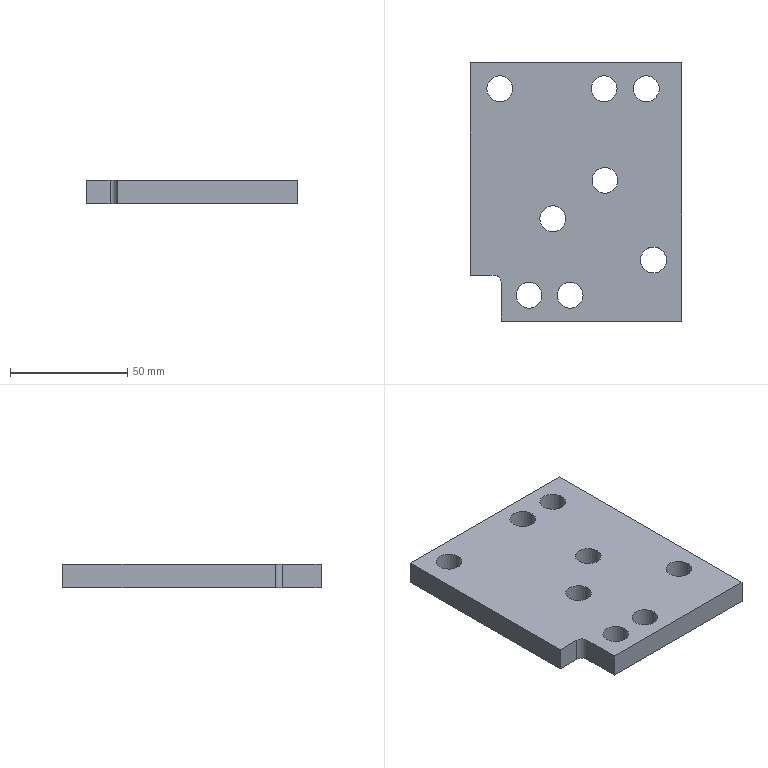Part | NX | features solid 2 | 1 solid | 17 faces | box 90 x 110 x 10 mm | volume 88862 mm3 | cylinder 9 | plane 8 | commonest cylinder face diameters 11 x8 6 x1
STEP:
#1=CARTESIAN_POINT('',(295.411,125.984,88.));
#2=VERTEX_POINT('',#1);
#3=CARTESIAN_POINT('',(295.411,15.984,88.));
#4=VERTEX_POINT('',#3);
#5=CARTESIAN_POINT('',(295.411,0.,88.));
#6=DIRECTION('',(0.,1.,0.));
#7=VECTOR('',#6,1000.);
#8=LINE('',#5,#7);
#9=EDGE_CURVE('',#2,#4,#8,.F.);
#10=ORIENTED_EDGE('',*,*,#9,.T.);
#11=CARTESIAN_POINT('',(295.411,15.984,78.));
#12=VERTEX_POINT('',#11);
#13=CARTESIAN_POINT('',(295.411,15.984,78.));
#14=DIRECTION('',(0.,0.,-1.));
#15=VECTOR('',#14,1000.);
#16=LINE('',#13,#15);
#17=EDGE_CURVE('',#12,#4,#16,.F.);
#18=ORIENTED_EDGE('',*,*,#17,.F.);
#19=CARTESIAN_POINT('',(295.411,125.984,78.));
#20=VERTEX_POINT('',#19);
#21=CARTESIAN_POINT('',(295.411,0.,78.));
#22=DIRECTION('',(0.,1.,0.));
#23=VECTOR('',#22,1000.);
#24=LINE('',#21,#23);
#25=EDGE_CURVE('',#20,#12,#24,.F.);
#26=ORIENTED_EDGE('',*,*,#25,.F.);
#27=CARTESIAN_POINT('',(295.411,125.984,78.));
#28=DIRECTION('',(0.,0.,-1.));
#29=VECTOR('',#28,1000.);
#30=LINE('',#27,#29);
#31=EDGE_CURVE('',#2,#20,#30,.T.);
#32=ORIENTED_EDGE('',*,*,#31,.F.);
#33=EDGE_LOOP('',(#10,#18,#26,#32));
#34=FACE_BOUND('',#33,.T.);
#35=CARTESIAN_POINT('',(295.411,71.771,78.));
#36=DIRECTION('',(-1.,0.,0.));
#37=DIRECTION('',(0.,1.,0.));
#38=AXIS2_PLACEMENT_3D('',#35,#36,#37);
#39=PLANE('',#38);
#40=ADVANCED_FACE('',(#34),#39,.F.);
#41=ORIENTED_EDGE('',*,*,#31,.T.);
#42=CARTESIAN_POINT('',(205.411,125.984,78.));
#43=VERTEX_POINT('',#42);
#44=CARTESIAN_POINT('',(247.131,125.984,78.));
#45=DIRECTION('',(-1.,0.,0.));
#46=VECTOR('',#45,1000.);
#47=LINE('',#44,#46);
#48=EDGE_CURVE('',#43,#20,#47,.F.);
#49=ORIENTED_EDGE('',*,*,#48,.F.);
#50=CARTESIAN_POINT('',(205.411,125.984,88.));
#51=VERTEX_POINT('',#50);
#52=CARTESIAN_POINT('',(205.411,125.984,78.));
#53=DIRECTION('',(0.,0.,1.));
#54=VECTOR('',#53,1000.);
#55=LINE('',#52,#54);
#56=EDGE_CURVE('',#51,#43,#55,.F.);
#57=ORIENTED_EDGE('',*,*,#56,.F.);
#58=CARTESIAN_POINT('',(188.,125.984,88.));
#59=DIRECTION('',(-1.,0.,0.));
#60=VECTOR('',#59,1000.);
#61=LINE('',#58,#60);
#62=EDGE_CURVE('',#51,#2,#61,.F.);
#63=ORIENTED_EDGE('',*,*,#62,.T.);
#64=EDGE_LOOP('',(#41,#49,#57,#63));
#65=FACE_BOUND('',#64,.T.);
#66=CARTESIAN_POINT('',(247.131,125.984,78.));
#67=DIRECTION('',(0.,-1.,0.));
#68=DIRECTION('',(-1.,0.,0.));
#69=AXIS2_PLACEMENT_3D('',#66,#67,#68);
#70=PLANE('',#69);
#71=ADVANCED_FACE('',(#65),#70,.F.);
#72=ORIENTED_EDGE('',*,*,#56,.T.);
#73=CARTESIAN_POINT('',(205.411,35.5,78.));
#74=VERTEX_POINT('',#73);
#75=CARTESIAN_POINT('',(205.411,71.771,78.));
#76=DIRECTION('',(0.,-1.,0.));
#77=VECTOR('',#76,1000.);
#78=LINE('',#75,#77);
#79=EDGE_CURVE('',#74,#43,#78,.F.);
#80=ORIENTED_EDGE('',*,*,#79,.F.);
#81=CARTESIAN_POINT('',(205.411,35.5,88.));
#82=VERTEX_POINT('',#81);
#83=CARTESIAN_POINT('',(205.411,35.5,78.));
#84=DIRECTION('',(0.,0.,1.));
#85=VECTOR('',#84,1000.);
#86=LINE('',#83,#85);
#87=EDGE_CURVE('',#82,#74,#86,.F.);
#88=ORIENTED_EDGE('',*,*,#87,.F.);
#89=CARTESIAN_POINT('',(205.411,0.,88.));
#90=DIRECTION('',(0.,1.,0.));
#91=VECTOR('',#90,1000.);
#92=LINE('',#89,#91);
#93=EDGE_CURVE('',#82,#51,#92,.T.);
#94=ORIENTED_EDGE('',*,*,#93,.T.);
#95=EDGE_LOOP('',(#72,#80,#88,#94));
#96=FACE_BOUND('',#95,.T.);
#97=CARTESIAN_POINT('',(205.411,71.771,78.));
#98=DIRECTION('',(1.,0.,0.));
#99=DIRECTION('',(0.,-1.,0.));
#100=AXIS2_PLACEMENT_3D('',#97,#98,#99);
#101=PLANE('',#100);
#102=ADVANCED_FACE('',(#96),#101,.F.);
#103=CARTESIAN_POINT('',(215.5,35.5,78.));
#104=VERTEX_POINT('',#103);
#105=CARTESIAN_POINT('',(188.,35.5,78.));
#106=DIRECTION('',(-1.,0.,0.));
#107=VECTOR('',#106,1000.);
#108=LINE('',#105,#107);
#109=EDGE_CURVE('',#104,#74,#108,.T.);
#110=ORIENTED_EDGE('',*,*,#109,.F.);
#111=CARTESIAN_POINT('',(215.5,35.5,88.));
#112=VERTEX_POINT('',#111);
#113=CARTESIAN_POINT('',(215.5,35.5,88.));
#114=DIRECTION('',(0.,0.,1.));
#115=VECTOR('',#114,1000.);
#116=LINE('',#113,#115);
#117=EDGE_CURVE('',#104,#112,#116,.T.);
#118=ORIENTED_EDGE('',*,*,#117,.T.);
#119=CARTESIAN_POINT('',(188.,35.5,88.));
#120=DIRECTION('',(-1.,0.,0.));
#121=VECTOR('',#120,1000.);
#122=LINE('',#119,#121);
#123=EDGE_CURVE('',#112,#82,#122,.T.);
#124=ORIENTED_EDGE('',*,*,#123,.T.);
#125=ORIENTED_EDGE('',*,*,#87,.T.);
#126=EDGE_LOOP('',(#110,#118,#124,#125));
#127=FACE_BOUND('',#126,.T.);
#128=CARTESIAN_POINT('',(188.,35.5,78.));
#129=DIRECTION('',(0.,-1.,0.));
#130=DIRECTION('',(-1.,0.,0.));
#131=AXIS2_PLACEMENT_3D('',#128,#129,#130);
#132=PLANE('',#131);
#133=ADVANCED_FACE('',(#127),#132,.T.);
#134=CARTESIAN_POINT('',(218.5,15.984,88.));
#135=VERTEX_POINT('',#134);
#136=CARTESIAN_POINT('',(218.5,32.5,88.));
#137=VERTEX_POINT('',#136);
#138=CARTESIAN_POINT('',(218.5,0.,88.));
#139=DIRECTION('',(0.,1.,0.));
#140=VECTOR('',#139,1000.);
#141=LINE('',#138,#140);
#142=EDGE_CURVE('',#135,#137,#141,.T.);
#143=ORIENTED_EDGE('',*,*,#142,.T.);
#144=CARTESIAN_POINT('',(218.5,32.5,78.));
#145=VERTEX_POINT('',#144);
#146=CARTESIAN_POINT('',(218.5,32.5,78.));
#147=DIRECTION('',(0.,0.,1.));
#148=VECTOR('',#147,1000.);
#149=LINE('',#146,#148);
#150=EDGE_CURVE('',#137,#145,#149,.F.);
#151=ORIENTED_EDGE('',*,*,#150,.T.);
#152=CARTESIAN_POINT('',(218.5,15.984,78.));
#153=VERTEX_POINT('',#152);
#154=CARTESIAN_POINT('',(218.5,0.,78.));
#155=DIRECTION('',(0.,1.,0.));
#156=VECTOR('',#155,1000.);
#157=LINE('',#154,#156);
#158=EDGE_CURVE('',#153,#145,#157,.T.);
#159=ORIENTED_EDGE('',*,*,#158,.F.);
#160=CARTESIAN_POINT('',(218.5,15.984,78.));
#161=DIRECTION('',(0.,0.,1.));
#162=VECTOR('',#161,1000.);
#163=LINE('',#160,#162);
#164=EDGE_CURVE('',#135,#153,#163,.F.);
#165=ORIENTED_EDGE('',*,*,#164,.F.);
#166=EDGE_LOOP('',(#143,#151,#159,#165));
#167=FACE_BOUND('',#166,.T.);
#168=CARTESIAN_POINT('',(218.5,0.,78.));
#169=DIRECTION('',(-1.,0.,0.));
#170=DIRECTION('',(0.,1.,0.));
#171=AXIS2_PLACEMENT_3D('',#168,#169,#170);
#172=PLANE('',#171);
#173=ADVANCED_FACE('',(#167),#172,.T.);
#174=CARTESIAN_POINT('',(242.411,26.984,78.));
#175=VERTEX_POINT('',#174);
#176=CARTESIAN_POINT('',(247.911,26.984,78.));
#177=DIRECTION('',(0.,0.,-1.));
#178=DIRECTION('',(-1.,0.,0.));
#179=AXIS2_PLACEMENT_3D('',#176,#177,#178);
#180=CIRCLE('',#179,5.5);
#181=EDGE_CURVE('',#175,#175,#180,.T.);
#182=ORIENTED_EDGE('',*,*,#181,.T.);
#183=EDGE_LOOP('',(#182));
#184=FACE_BOUND('',#183,.T.);
#185=CARTESIAN_POINT('',(242.411,26.984,88.));
#186=VERTEX_POINT('',#185);
#187=CARTESIAN_POINT('',(247.911,26.984,88.));
#188=DIRECTION('',(0.,0.,-1.));
#189=DIRECTION('',(-1.,0.,0.));
#190=AXIS2_PLACEMENT_3D('',#187,#188,#189);
#191=CIRCLE('',#190,5.5);
#192=EDGE_CURVE('',#186,#186,#191,.T.);
#193=ORIENTED_EDGE('',*,*,#192,.F.);
#194=EDGE_LOOP('',(#193));
#195=FACE_BOUND('',#194,.T.);
#196=CARTESIAN_POINT('',(247.911,26.984,78.));
#197=DIRECTION('',(0.,0.,-1.));
#198=DIRECTION('',(-1.,0.,0.));
#199=AXIS2_PLACEMENT_3D('',#196,#197,#198);
#200=CYLINDRICAL_SURFACE('',#199,5.5);
#201=ADVANCED_FACE('',(#184,#195),#200,.F.);
#202=CARTESIAN_POINT('',(256.911,114.984,78.));
#203=VERTEX_POINT('',#202);
#204=CARTESIAN_POINT('',(262.411,114.984,78.));
#205=DIRECTION('',(0.,0.,-1.));
#206=DIRECTION('',(-1.,0.,0.));
#207=AXIS2_PLACEMENT_3D('',#204,#205,#206);
#208=CIRCLE('',#207,5.5);
#209=EDGE_CURVE('',#203,#203,#208,.F.);
#210=ORIENTED_EDGE('',*,*,#209,.F.);
#211=EDGE_LOOP('',(#210));
#212=FACE_BOUND('',#211,.T.);
#213=CARTESIAN_POINT('',(256.911,114.984,88.));
#214=VERTEX_POINT('',#213);
#215=CARTESIAN_POINT('',(262.411,114.984,88.));
#216=DIRECTION('',(0.,0.,-1.));
#217=DIRECTION('',(-1.,0.,0.));
#218=AXIS2_PLACEMENT_3D('',#215,#216,#217);
#219=CIRCLE('',#218,5.5);
#220=EDGE_CURVE('',#214,#214,#219,.F.);
#221=ORIENTED_EDGE('',*,*,#220,.T.);
#222=EDGE_LOOP('',(#221));
#223=FACE_BOUND('',#222,.T.);
#224=CARTESIAN_POINT('',(262.411,114.984,78.));
#225=DIRECTION('',(0.,0.,-1.));
#226=DIRECTION('',(-1.,0.,0.));
#227=AXIS2_PLACEMENT_3D('',#224,#225,#226);
#228=CYLINDRICAL_SURFACE('',#227,5.5);
#229=ADVANCED_FACE('',(#212,#223),#228,.F.);
#230=CARTESIAN_POINT('',(247.131,15.984,78.));
#231=DIRECTION('',(1.,0.,0.));
#232=VECTOR('',#231,1000.);
#233=LINE('',#230,#232);
#234=EDGE_CURVE('',#12,#153,#233,.F.);
#235=ORIENTED_EDGE('',*,*,#234,.F.);
#236=ORIENTED_EDGE('',*,*,#17,.T.);
#237=CARTESIAN_POINT('',(188.,15.984,88.));
#238=DIRECTION('',(-1.,0.,0.));
#239=VECTOR('',#238,1000.);
#240=LINE('',#237,#239);
#241=EDGE_CURVE('',#4,#135,#240,.T.);
#242=ORIENTED_EDGE('',*,*,#241,.T.);
#243=ORIENTED_EDGE('',*,*,#164,.T.);
#244=EDGE_LOOP('',(#235,#236,#242,#243));
#245=FACE_BOUND('',#244,.T.);
#246=CARTESIAN_POINT('',(247.131,15.984,78.));
#247=DIRECTION('',(0.,1.,0.));
#248=DIRECTION('',(1.,0.,0.));
#249=AXIS2_PLACEMENT_3D('',#246,#247,#248);
#250=PLANE('',#249);
#251=ADVANCED_FACE('',(#245),#250,.F.);
#252=CARTESIAN_POINT('',(212.411,114.984,78.));
#253=VERTEX_POINT('',#252);
#254=CARTESIAN_POINT('',(217.911,114.984,78.));
#255=DIRECTION('',(0.,0.,-1.));
#256=DIRECTION('',(-1.,0.,0.));
#257=AXIS2_PLACEMENT_3D('',#254,#255,#256);
#258=CIRCLE('',#257,5.5);
#259=EDGE_CURVE('',#253,#253,#258,.T.);
#260=ORIENTED_EDGE('',*,*,#259,.T.);
#261=EDGE_LOOP('',(#260));
#262=FACE_BOUND('',#261,.T.);
#263=CARTESIAN_POINT('',(212.411,114.984,88.));
#264=VERTEX_POINT('',#263);
#265=CARTESIAN_POINT('',(217.911,114.984,88.));
#266=DIRECTION('',(0.,0.,-1.));
#267=DIRECTION('',(-1.,0.,0.));
#268=AXIS2_PLACEMENT_3D('',#265,#266,#267);
#269=CIRCLE('',#268,5.5);
#270=EDGE_CURVE('',#264,#264,#269,.T.);
#271=ORIENTED_EDGE('',*,*,#270,.F.);
#272=EDGE_LOOP('',(#271));
#273=FACE_BOUND('',#272,.T.);
#274=CARTESIAN_POINT('',(217.911,114.984,78.));
#275=DIRECTION('',(0.,0.,-1.));
#276=DIRECTION('',(-1.,0.,0.));
#277=AXIS2_PLACEMENT_3D('',#274,#275,#276);
#278=CYLINDRICAL_SURFACE('',#277,5.5);
#279=ADVANCED_FACE('',(#262,#273),#278,.F.);
#280=CARTESIAN_POINT('',(274.911,114.984,78.));
#281=VERTEX_POINT('',#280);
#282=CARTESIAN_POINT('',(280.411,114.984,78.));
#283=DIRECTION('',(0.,0.,-1.));
#284=DIRECTION('',(-1.,0.,0.));
#285=AXIS2_PLACEMENT_3D('',#282,#283,#284);
#286=CIRCLE('',#285,5.5);
#287=EDGE_CURVE('',#281,#281,#286,.T.);
#288=ORIENTED_EDGE('',*,*,#287,.T.);
#289=EDGE_LOOP('',(#288));
#290=FACE_BOUND('',#289,.T.);
#291=CARTESIAN_POINT('',(274.911,114.984,88.));
#292=VERTEX_POINT('',#291);
#293=CARTESIAN_POINT('',(280.411,114.984,88.));
#294=DIRECTION('',(0.,0.,-1.));
#295=DIRECTION('',(-1.,0.,0.));
#296=AXIS2_PLACEMENT_3D('',#293,#294,#295);
#297=CIRCLE('',#296,5.5);
#298=EDGE_CURVE('',#292,#292,#297,.T.);
#299=ORIENTED_EDGE('',*,*,#298,.F.);
#300=EDGE_LOOP('',(#299));
#301=FACE_BOUND('',#300,.T.);
#302=CARTESIAN_POINT('',(280.411,114.984,78.));
#303=DIRECTION('',(0.,0.,-1.));
#304=DIRECTION('',(-1.,0.,0.));
#305=AXIS2_PLACEMENT_3D('',#302,#303,#304);
#306=CYLINDRICAL_SURFACE('',#305,5.5);
#307=ADVANCED_FACE('',(#290,#301),#306,.F.);
#308=CARTESIAN_POINT('',(277.911,41.984,78.));
#309=VERTEX_POINT('',#308);
#310=CARTESIAN_POINT('',(283.411,41.984,78.));
#311=DIRECTION('',(0.,0.,-1.));
#312=DIRECTION('',(-1.,0.,0.));
#313=AXIS2_PLACEMENT_3D('',#310,#311,#312);
#314=CIRCLE('',#313,5.5);
#315=EDGE_CURVE('',#309,#309,#314,.F.);
#316=ORIENTED_EDGE('',*,*,#315,.F.);
#317=EDGE_LOOP('',(#316));
#318=FACE_BOUND('',#317,.T.);
#319=CARTESIAN_POINT('',(277.911,41.984,88.));
#320=VERTEX_POINT('',#319);
#321=CARTESIAN_POINT('',(283.411,41.984,88.));
#322=DIRECTION('',(0.,0.,-1.));
#323=DIRECTION('',(-1.,0.,0.));
#324=AXIS2_PLACEMENT_3D('',#321,#322,#323);
#325=CIRCLE('',#324,5.5);
#326=EDGE_CURVE('',#320,#320,#325,.F.);
#327=ORIENTED_EDGE('',*,*,#326,.T.);
#328=EDGE_LOOP('',(#327));
#329=FACE_BOUND('',#328,.T.);
#330=CARTESIAN_POINT('',(283.411,41.984,78.));
#331=DIRECTION('',(0.,0.,-1.));
#332=DIRECTION('',(-1.,0.,0.));
#333=AXIS2_PLACEMENT_3D('',#330,#331,#332);
#334=CYLINDRICAL_SURFACE('',#333,5.5);
#335=ADVANCED_FACE('',(#318,#329),#334,.F.);
#336=CARTESIAN_POINT('',(224.911,26.984,78.));
#337=VERTEX_POINT('',#336);
#338=CARTESIAN_POINT('',(230.411,26.984,78.));
#339=DIRECTION('',(0.,0.,-1.));
#340=DIRECTION('',(-1.,0.,0.));
#341=AXIS2_PLACEMENT_3D('',#338,#339,#340);
#342=CIRCLE('',#341,5.5);
#343=EDGE_CURVE('',#337,#337,#342,.F.);
#344=ORIENTED_EDGE('',*,*,#343,.F.);
#345=EDGE_LOOP('',(#344));
#346=FACE_BOUND('',#345,.T.);
#347=CARTESIAN_POINT('',(224.911,26.984,88.));
#348=VERTEX_POINT('',#347);
#349=CARTESIAN_POINT('',(230.411,26.984,88.));
#350=DIRECTION('',(0.,0.,-1.));
#351=DIRECTION('',(-1.,0.,0.));
#352=AXIS2_PLACEMENT_3D('',#349,#350,#351);
#353=CIRCLE('',#352,5.5);
#354=EDGE_CURVE('',#348,#348,#353,.F.);
#355=ORIENTED_EDGE('',*,*,#354,.T.);
#356=EDGE_LOOP('',(#355));
#357=FACE_BOUND('',#356,.T.);
#358=CARTESIAN_POINT('',(230.411,26.984,78.));
#359=DIRECTION('',(0.,0.,-1.));
#360=DIRECTION('',(-1.,0.,0.));
#361=AXIS2_PLACEMENT_3D('',#358,#359,#360);
#362=CYLINDRICAL_SURFACE('',#361,5.5);
#363=ADVANCED_FACE('',(#346,#357),#362,.F.);
#364=CARTESIAN_POINT('',(257.24,75.929,78.));
#365=VERTEX_POINT('',#364);
#366=CARTESIAN_POINT('',(262.74,75.929,78.));
#367=DIRECTION('',(0.,0.,-1.));
#368=DIRECTION('',(-1.,0.,0.));
#369=AXIS2_PLACEMENT_3D('',#366,#367,#368);
#370=CIRCLE('',#369,5.5);
#371=EDGE_CURVE('',#365,#365,#370,.F.);
#372=ORIENTED_EDGE('',*,*,#371,.F.);
#373=EDGE_LOOP('',(#372));
#374=FACE_BOUND('',#373,.T.);
#375=CARTESIAN_POINT('',(257.24,75.929,88.));
#376=VERTEX_POINT('',#375);
#377=CARTESIAN_POINT('',(262.74,75.929,88.));
#378=DIRECTION('',(0.,0.,-1.));
#379=DIRECTION('',(-1.,0.,0.));
#380=AXIS2_PLACEMENT_3D('',#377,#378,#379);
#381=CIRCLE('',#380,5.5);
#382=EDGE_CURVE('',#376,#376,#381,.F.);
#383=ORIENTED_EDGE('',*,*,#382,.T.);
#384=EDGE_LOOP('',(#383));
#385=FACE_BOUND('',#384,.T.);
#386=CARTESIAN_POINT('',(262.74,75.929,78.));
#387=DIRECTION('',(0.,0.,-1.));
#388=DIRECTION('',(-1.,0.,0.));
#389=AXIS2_PLACEMENT_3D('',#386,#387,#388);
#390=CYLINDRICAL_SURFACE('',#389,5.5);
#391=ADVANCED_FACE('',(#374,#385),#390,.F.);
#392=CARTESIAN_POINT('',(235.001,59.571,78.));
#393=VERTEX_POINT('',#392);
#394=CARTESIAN_POINT('',(240.501,59.571,78.));
#395=DIRECTION('',(0.,0.,-1.));
#396=DIRECTION('',(-1.,0.,0.));
#397=AXIS2_PLACEMENT_3D('',#394,#395,#396);
#398=CIRCLE('',#397,5.5);
#399=EDGE_CURVE('',#393,#393,#398,.T.);
#400=ORIENTED_EDGE('',*,*,#399,.T.);
#401=EDGE_LOOP('',(#400));
#402=FACE_BOUND('',#401,.T.);
#403=CARTESIAN_POINT('',(235.001,59.571,88.));
#404=VERTEX_POINT('',#403);
#405=CARTESIAN_POINT('',(240.501,59.571,88.));
#406=DIRECTION('',(0.,0.,-1.));
#407=DIRECTION('',(-1.,0.,0.));
#408=AXIS2_PLACEMENT_3D('',#405,#406,#407);
#409=CIRCLE('',#408,5.5);
#410=EDGE_CURVE('',#404,#404,#409,.T.);
#411=ORIENTED_EDGE('',*,*,#410,.F.);
#412=EDGE_LOOP('',(#411));
#413=FACE_BOUND('',#412,.T.);
#414=CARTESIAN_POINT('',(240.501,59.571,78.));
#415=DIRECTION('',(0.,0.,-1.));
#416=DIRECTION('',(-1.,0.,0.));
#417=AXIS2_PLACEMENT_3D('',#414,#415,#416);
#418=CYLINDRICAL_SURFACE('',#417,5.5);
#419=ADVANCED_FACE('',(#402,#413),#418,.F.);
#420=ORIENTED_EDGE('',*,*,#25,.T.);
#421=ORIENTED_EDGE('',*,*,#234,.T.);
#422=ORIENTED_EDGE('',*,*,#158,.T.);
#423=CARTESIAN_POINT('',(215.5,32.5,78.));
#424=DIRECTION('',(0.,0.,-1.));
#425=DIRECTION('',(-1.,0.,0.));
#426=AXIS2_PLACEMENT_3D('',#423,#424,#425);
#427=CIRCLE('',#426,3.);
#428=EDGE_CURVE('',#145,#104,#427,.F.);
#429=ORIENTED_EDGE('',*,*,#428,.T.);
#430=ORIENTED_EDGE('',*,*,#109,.T.);
#431=ORIENTED_EDGE('',*,*,#79,.T.);
#432=ORIENTED_EDGE('',*,*,#48,.T.);
#433=EDGE_LOOP('',(#420,#421,#422,#429,#430,#431,#432));
#434=FACE_BOUND('',#433,.T.);
#435=ORIENTED_EDGE('',*,*,#371,.T.);
#436=EDGE_LOOP('',(#435));
#437=FACE_BOUND('',#436,.T.);
#438=ORIENTED_EDGE('',*,*,#399,.F.);
#439=EDGE_LOOP('',(#438));
#440=FACE_BOUND('',#439,.T.);
#441=ORIENTED_EDGE('',*,*,#181,.F.);
#442=EDGE_LOOP('',(#441));
#443=FACE_BOUND('',#442,.T.);
#444=ORIENTED_EDGE('',*,*,#209,.T.);
#445=EDGE_LOOP('',(#444));
#446=FACE_BOUND('',#445,.T.);
#447=ORIENTED_EDGE('',*,*,#259,.F.);
#448=EDGE_LOOP('',(#447));
#449=FACE_BOUND('',#448,.T.);
#450=ORIENTED_EDGE('',*,*,#287,.F.);
#451=EDGE_LOOP('',(#450));
#452=FACE_BOUND('',#451,.T.);
#453=ORIENTED_EDGE('',*,*,#315,.T.);
#454=EDGE_LOOP('',(#453));
#455=FACE_BOUND('',#454,.T.);
#456=ORIENTED_EDGE('',*,*,#343,.T.);
#457=EDGE_LOOP('',(#456));
#458=FACE_BOUND('',#457,.T.);
#459=CARTESIAN_POINT('',(188.,0.,78.));
#460=DIRECTION('',(0.,0.,-1.));
#461=DIRECTION('',(-1.,0.,0.));
#462=AXIS2_PLACEMENT_3D('',#459,#460,#461);
#463=PLANE('',#462);
#464=ADVANCED_FACE('',(#434,#437,#440,#443,#446,#449,#452,#455,#458),#463,.T.);
#465=ORIENTED_EDGE('',*,*,#241,.F.);
#466=ORIENTED_EDGE('',*,*,#9,.F.);
#467=ORIENTED_EDGE('',*,*,#62,.F.);
#468=ORIENTED_EDGE('',*,*,#93,.F.);
#469=ORIENTED_EDGE('',*,*,#123,.F.);
#470=CARTESIAN_POINT('',(215.5,32.5,88.));
#471=DIRECTION('',(0.,0.,-1.));
#472=DIRECTION('',(-1.,0.,0.));
#473=AXIS2_PLACEMENT_3D('',#470,#471,#472);
#474=CIRCLE('',#473,3.);
#475=EDGE_CURVE('',#112,#137,#474,.T.);
#476=ORIENTED_EDGE('',*,*,#475,.T.);
#477=ORIENTED_EDGE('',*,*,#142,.F.);
#478=EDGE_LOOP('',(#465,#466,#467,#468,#469,#476,#477));
#479=FACE_BOUND('',#478,.T.);
#480=ORIENTED_EDGE('',*,*,#382,.F.);
#481=EDGE_LOOP('',(#480));
#482=FACE_BOUND('',#481,.T.);
#483=ORIENTED_EDGE('',*,*,#410,.T.);
#484=EDGE_LOOP('',(#483));
#485=FACE_BOUND('',#484,.T.);
#486=ORIENTED_EDGE('',*,*,#192,.T.);
#487=EDGE_LOOP('',(#486));
#488=FACE_BOUND('',#487,.T.);
#489=ORIENTED_EDGE('',*,*,#220,.F.);
#490=EDGE_LOOP('',(#489));
#491=FACE_BOUND('',#490,.T.);
#492=ORIENTED_EDGE('',*,*,#270,.T.);
#493=EDGE_LOOP('',(#492));
#494=FACE_BOUND('',#493,.T.);
#495=ORIENTED_EDGE('',*,*,#298,.T.);
#496=EDGE_LOOP('',(#495));
#497=FACE_BOUND('',#496,.T.);
#498=ORIENTED_EDGE('',*,*,#326,.F.);
#499=EDGE_LOOP('',(#498));
#500=FACE_BOUND('',#499,.T.);
#501=ORIENTED_EDGE('',*,*,#354,.F.);
#502=EDGE_LOOP('',(#501));
#503=FACE_BOUND('',#502,.T.);
#504=CARTESIAN_POINT('',(188.,0.,88.));
#505=DIRECTION('',(0.,0.,-1.));
#506=DIRECTION('',(-1.,0.,0.));
#507=AXIS2_PLACEMENT_3D('',#504,#505,#506);
#508=PLANE('',#507);
#509=ADVANCED_FACE('',(#479,#482,#485,#488,#491,#494,#497,#500,#503),#508,.F.);
#510=ORIENTED_EDGE('',*,*,#475,.F.);
#511=ORIENTED_EDGE('',*,*,#117,.F.);
#512=ORIENTED_EDGE('',*,*,#428,.F.);
#513=ORIENTED_EDGE('',*,*,#150,.F.);
#514=EDGE_LOOP('',(#510,#511,#512,#513));
#515=FACE_BOUND('',#514,.T.);
#516=CARTESIAN_POINT('',(215.5,32.5,78.));
#517=DIRECTION('',(0.,0.,1.));
#518=DIRECTION('',(1.,0.,0.));
#519=AXIS2_PLACEMENT_3D('',#516,#517,#518);
#520=CYLINDRICAL_SURFACE('',#519,3.);
#521=ADVANCED_FACE('',(#515),#520,.F.);
#522=CLOSED_SHELL('',(#40,#71,#102,#133,#173,#201,#229,#251,#279,#307,#335,#363,#391,#419,#464,#509,#521));
#523=MANIFOLD_SOLID_BREP('',#522);
#524=(LENGTH_UNIT()NAMED_UNIT(*)SI_UNIT(.MILLI.,.METRE.));
#525=UNCERTAINTY_MEASURE_WITH_UNIT(LENGTH_MEASURE(0.00001),#524,'','');
#526=(NAMED_UNIT(*)PLANE_ANGLE_UNIT()SI_UNIT($,.RADIAN.));
#527=(NAMED_UNIT(*)SI_UNIT($,.STERADIAN.)SOLID_ANGLE_UNIT());
#528=(GEOMETRIC_REPRESENTATION_CONTEXT(3)GLOBAL_UNCERTAINTY_ASSIGNED_CONTEXT((#525))GLOBAL_UNIT_ASSIGNED_CONTEXT((#524,#526,#527))REPRESENTATION_CONTEXT('',''));
#529=ADVANCED_BREP_SHAPE_REPRESENTATION('',(#523),#528);